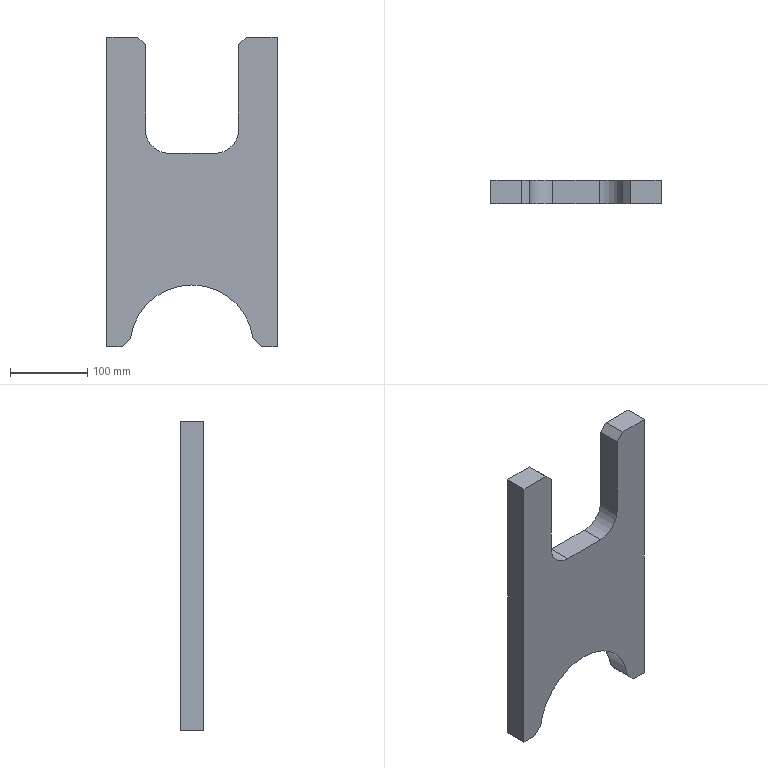Part | SolidWorks | features Chamfer 1, Extrusion 1, Fillet 1 | 1 solid | 18 faces | box 220 x 30 x 400 mm | volume 1803857 mm3 | plane 15 | cylinder 3 | commonest cylinder face diameters 60 x2 160 x1
STEP:
#1=CARTESIAN_POINT('',(110.,0.,200.));
#2=VERTEX_POINT('',#1);
#3=CARTESIAN_POINT('',(110.,0.,-200.));
#4=VERTEX_POINT('',#3);
#5=CARTESIAN_POINT('',(110.,0.,200.));
#6=DIRECTION('',(0.,0.,-1.));
#7=VECTOR('',#6,1000.);
#8=LINE('',#5,#7);
#9=EDGE_CURVE('',#2,#4,#8,.T.);
#10=ORIENTED_EDGE('',*,*,#9,.T.);
#11=CARTESIAN_POINT('',(110.,30.,-200.));
#12=VERTEX_POINT('',#11);
#13=CARTESIAN_POINT('',(110.,30.,-200.));
#14=DIRECTION('',(0.,-1.,0.));
#15=VECTOR('',#14,1000.);
#16=LINE('',#13,#15);
#17=EDGE_CURVE('',#12,#4,#16,.T.);
#18=ORIENTED_EDGE('',*,*,#17,.F.);
#19=CARTESIAN_POINT('',(110.,30.,200.));
#20=VERTEX_POINT('',#19);
#21=CARTESIAN_POINT('',(110.,30.,200.));
#22=DIRECTION('',(0.,0.,-1.));
#23=VECTOR('',#22,1000.);
#24=LINE('',#21,#23);
#25=EDGE_CURVE('',#20,#12,#24,.T.);
#26=ORIENTED_EDGE('',*,*,#25,.F.);
#27=CARTESIAN_POINT('',(110.,30.,200.));
#28=DIRECTION('',(0.,-1.,0.));
#29=VECTOR('',#28,1000.);
#30=LINE('',#27,#29);
#31=EDGE_CURVE('',#20,#2,#30,.T.);
#32=ORIENTED_EDGE('',*,*,#31,.T.);
#33=EDGE_LOOP('',(#10,#18,#26,#32));
#34=FACE_OUTER_BOUND('',#33,.T.);
#35=CARTESIAN_POINT('',(110.,30.,200.));
#36=DIRECTION('',(-1.,0.,0.));
#37=DIRECTION('',(0.,0.,1.));
#38=AXIS2_PLACEMENT_3D('',#35,#36,#37);
#39=PLANE('',#38);
#40=ADVANCED_FACE('',(#34),#39,.F.);
#41=CARTESIAN_POINT('',(89.703,0.,-200.));
#42=VERTEX_POINT('',#41);
#43=CARTESIAN_POINT('',(79.703,0.,-200.));
#44=DIRECTION('',(-1.,0.,0.));
#45=VECTOR('',#44,1000.);
#46=LINE('',#43,#45);
#47=EDGE_CURVE('',#4,#42,#46,.T.);
#48=ORIENTED_EDGE('',*,*,#47,.T.);
#49=CARTESIAN_POINT('',(89.703,30.,-200.));
#50=VERTEX_POINT('',#49);
#51=CARTESIAN_POINT('',(89.703,30.,-200.));
#52=DIRECTION('',(0.,1.,0.));
#53=VECTOR('',#52,1000.);
#54=LINE('',#51,#53);
#55=EDGE_CURVE('',#42,#50,#54,.T.);
#56=ORIENTED_EDGE('',*,*,#55,.T.);
#57=CARTESIAN_POINT('',(79.703,30.,-200.));
#58=DIRECTION('',(-1.,0.,0.));
#59=VECTOR('',#58,1000.);
#60=LINE('',#57,#59);
#61=EDGE_CURVE('',#12,#50,#60,.T.);
#62=ORIENTED_EDGE('',*,*,#61,.F.);
#63=ORIENTED_EDGE('',*,*,#17,.T.);
#64=EDGE_LOOP('',(#48,#56,#62,#63));
#65=FACE_OUTER_BOUND('',#64,.T.);
#66=CARTESIAN_POINT('',(79.703,30.,-200.));
#67=DIRECTION('',(0.,0.,1.));
#68=DIRECTION('',(1.,0.,0.));
#69=AXIS2_PLACEMENT_3D('',#66,#67,#68);
#70=PLANE('',#69);
#71=ADVANCED_FACE('',(#65),#70,.F.);
#72=CARTESIAN_POINT('',(78.981,30.,-189.278));
#73=VERTEX_POINT('',#72);
#74=CARTESIAN_POINT('',(-79.575,30.,-189.278));
#75=VERTEX_POINT('',#74);
#76=CARTESIAN_POINT('',(-0.2969,30.,-200.));
#77=DIRECTION('',(0.,-1.,0.));
#78=DIRECTION('',(0.,0.,1.));
#79=AXIS2_PLACEMENT_3D('',#76,#77,#78);
#80=CIRCLE('',#79,80.);
#81=EDGE_CURVE('',#73,#75,#80,.T.);
#82=ORIENTED_EDGE('',*,*,#81,.F.);
#83=CARTESIAN_POINT('',(78.981,0.,-189.278));
#84=VERTEX_POINT('',#83);
#85=CARTESIAN_POINT('',(78.981,30.,-189.278));
#86=DIRECTION('',(0.,-1.,0.));
#87=VECTOR('',#86,1000.);
#88=LINE('',#85,#87);
#89=EDGE_CURVE('',#73,#84,#88,.T.);
#90=ORIENTED_EDGE('',*,*,#89,.T.);
#91=CARTESIAN_POINT('',(-79.575,0.,-189.278));
#92=VERTEX_POINT('',#91);
#93=CARTESIAN_POINT('',(-0.2969,0.,-200.));
#94=DIRECTION('',(0.,-1.,0.));
#95=DIRECTION('',(0.,0.,1.));
#96=AXIS2_PLACEMENT_3D('',#93,#94,#95);
#97=CIRCLE('',#96,80.);
#98=EDGE_CURVE('',#84,#92,#97,.T.);
#99=ORIENTED_EDGE('',*,*,#98,.T.);
#100=CARTESIAN_POINT('',(-79.575,30.,-189.278));
#101=DIRECTION('',(0.,1.,0.));
#102=VECTOR('',#101,1000.);
#103=LINE('',#100,#102);
#104=EDGE_CURVE('',#92,#75,#103,.T.);
#105=ORIENTED_EDGE('',*,*,#104,.T.);
#106=EDGE_LOOP('',(#82,#90,#99,#105));
#107=FACE_OUTER_BOUND('',#106,.T.);
#108=CARTESIAN_POINT('',(-0.2969,30.,-200.));
#109=DIRECTION('',(0.,-1.,0.));
#110=DIRECTION('',(0.,0.,-1.));
#111=AXIS2_PLACEMENT_3D('',#108,#109,#110);
#112=CYLINDRICAL_SURFACE('',#111,80.);
#113=ADVANCED_FACE('',(#107),#112,.F.);
#114=CARTESIAN_POINT('',(-90.297,30.,-200.));
#115=VERTEX_POINT('',#114);
#116=CARTESIAN_POINT('',(-110.,30.,-200.));
#117=VERTEX_POINT('',#116);
#118=CARTESIAN_POINT('',(-110.,30.,-200.));
#119=DIRECTION('',(-1.,0.,0.));
#120=VECTOR('',#119,1000.);
#121=LINE('',#118,#120);
#122=EDGE_CURVE('',#115,#117,#121,.T.);
#123=ORIENTED_EDGE('',*,*,#122,.F.);
#124=CARTESIAN_POINT('',(-90.297,0.,-200.));
#125=VERTEX_POINT('',#124);
#126=CARTESIAN_POINT('',(-90.297,30.,-200.));
#127=DIRECTION('',(0.,-1.,0.));
#128=VECTOR('',#127,1000.);
#129=LINE('',#126,#128);
#130=EDGE_CURVE('',#115,#125,#129,.T.);
#131=ORIENTED_EDGE('',*,*,#130,.T.);
#132=CARTESIAN_POINT('',(-110.,0.,-200.));
#133=VERTEX_POINT('',#132);
#134=CARTESIAN_POINT('',(-110.,0.,-200.));
#135=DIRECTION('',(-1.,0.,0.));
#136=VECTOR('',#135,1000.);
#137=LINE('',#134,#136);
#138=EDGE_CURVE('',#125,#133,#137,.T.);
#139=ORIENTED_EDGE('',*,*,#138,.T.);
#140=CARTESIAN_POINT('',(-110.,30.,-200.));
#141=DIRECTION('',(0.,-1.,0.));
#142=VECTOR('',#141,1000.);
#143=LINE('',#140,#142);
#144=EDGE_CURVE('',#117,#133,#143,.T.);
#145=ORIENTED_EDGE('',*,*,#144,.F.);
#146=EDGE_LOOP('',(#123,#131,#139,#145));
#147=FACE_OUTER_BOUND('',#146,.T.);
#148=CARTESIAN_POINT('',(-110.,30.,-200.));
#149=DIRECTION('',(0.,0.,1.));
#150=DIRECTION('',(1.,0.,0.));
#151=AXIS2_PLACEMENT_3D('',#148,#149,#150);
#152=PLANE('',#151);
#153=ADVANCED_FACE('',(#147),#152,.F.);
#154=CARTESIAN_POINT('',(-110.,0.,200.));
#155=VERTEX_POINT('',#154);
#156=CARTESIAN_POINT('',(-110.,0.,200.));
#157=DIRECTION('',(0.,0.,1.));
#158=VECTOR('',#157,1000.);
#159=LINE('',#156,#158);
#160=EDGE_CURVE('',#133,#155,#159,.T.);
#161=ORIENTED_EDGE('',*,*,#160,.T.);
#162=CARTESIAN_POINT('',(-110.,30.,200.));
#163=VERTEX_POINT('',#162);
#164=CARTESIAN_POINT('',(-110.,30.,200.));
#165=DIRECTION('',(0.,-1.,0.));
#166=VECTOR('',#165,1000.);
#167=LINE('',#164,#166);
#168=EDGE_CURVE('',#163,#155,#167,.T.);
#169=ORIENTED_EDGE('',*,*,#168,.F.);
#170=CARTESIAN_POINT('',(-110.,30.,200.));
#171=DIRECTION('',(0.,0.,1.));
#172=VECTOR('',#171,1000.);
#173=LINE('',#170,#172);
#174=EDGE_CURVE('',#117,#163,#173,.T.);
#175=ORIENTED_EDGE('',*,*,#174,.F.);
#176=ORIENTED_EDGE('',*,*,#144,.T.);
#177=EDGE_LOOP('',(#161,#169,#175,#176));
#178=FACE_OUTER_BOUND('',#177,.T.);
#179=CARTESIAN_POINT('',(-110.,30.,200.));
#180=DIRECTION('',(1.,0.,0.));
#181=DIRECTION('',(0.,0.,-1.));
#182=AXIS2_PLACEMENT_3D('',#179,#180,#181);
#183=PLANE('',#182);
#184=ADVANCED_FACE('',(#178),#183,.F.);
#185=CARTESIAN_POINT('',(-70.,0.,200.));
#186=VERTEX_POINT('',#185);
#187=CARTESIAN_POINT('',(-110.,0.,200.));
#188=DIRECTION('',(1.,0.,0.));
#189=VECTOR('',#188,1000.);
#190=LINE('',#187,#189);
#191=EDGE_CURVE('',#155,#186,#190,.T.);
#192=ORIENTED_EDGE('',*,*,#191,.T.);
#193=CARTESIAN_POINT('',(-70.,30.,200.));
#194=VERTEX_POINT('',#193);
#195=CARTESIAN_POINT('',(-70.,30.,200.));
#196=DIRECTION('',(0.,1.,0.));
#197=VECTOR('',#196,1000.);
#198=LINE('',#195,#197);
#199=EDGE_CURVE('',#186,#194,#198,.T.);
#200=ORIENTED_EDGE('',*,*,#199,.T.);
#201=CARTESIAN_POINT('',(-110.,30.,200.));
#202=DIRECTION('',(1.,0.,0.));
#203=VECTOR('',#202,1000.);
#204=LINE('',#201,#203);
#205=EDGE_CURVE('',#163,#194,#204,.T.);
#206=ORIENTED_EDGE('',*,*,#205,.F.);
#207=ORIENTED_EDGE('',*,*,#168,.T.);
#208=EDGE_LOOP('',(#192,#200,#206,#207));
#209=FACE_OUTER_BOUND('',#208,.T.);
#210=CARTESIAN_POINT('',(-110.,30.,200.));
#211=DIRECTION('',(0.,0.,-1.));
#212=DIRECTION('',(-1.,0.,0.));
#213=AXIS2_PLACEMENT_3D('',#210,#211,#212);
#214=PLANE('',#213);
#215=ADVANCED_FACE('',(#209),#214,.F.);
#216=CARTESIAN_POINT('',(-60.,30.,190.));
#217=VERTEX_POINT('',#216);
#218=CARTESIAN_POINT('',(-60.,30.,80.));
#219=VERTEX_POINT('',#218);
#220=CARTESIAN_POINT('',(-60.,30.,200.));
#221=DIRECTION('',(0.,0.,-1.));
#222=VECTOR('',#221,1000.);
#223=LINE('',#220,#222);
#224=EDGE_CURVE('',#217,#219,#223,.T.);
#225=ORIENTED_EDGE('',*,*,#224,.F.);
#226=CARTESIAN_POINT('',(-60.,0.,190.));
#227=VERTEX_POINT('',#226);
#228=CARTESIAN_POINT('',(-60.,30.,190.));
#229=DIRECTION('',(0.,-1.,0.));
#230=VECTOR('',#229,1000.);
#231=LINE('',#228,#230);
#232=EDGE_CURVE('',#217,#227,#231,.T.);
#233=ORIENTED_EDGE('',*,*,#232,.T.);
#234=CARTESIAN_POINT('',(-60.,0.,80.));
#235=VERTEX_POINT('',#234);
#236=CARTESIAN_POINT('',(-60.,0.,200.));
#237=DIRECTION('',(0.,0.,-1.));
#238=VECTOR('',#237,1000.);
#239=LINE('',#236,#238);
#240=EDGE_CURVE('',#227,#235,#239,.T.);
#241=ORIENTED_EDGE('',*,*,#240,.T.);
#242=CARTESIAN_POINT('',(-60.,30.,80.));
#243=DIRECTION('',(0.,1.,0.));
#244=VECTOR('',#243,1000.);
#245=LINE('',#242,#244);
#246=EDGE_CURVE('',#235,#219,#245,.T.);
#247=ORIENTED_EDGE('',*,*,#246,.T.);
#248=EDGE_LOOP('',(#225,#233,#241,#247));
#249=FACE_OUTER_BOUND('',#248,.T.);
#250=CARTESIAN_POINT('',(-60.,30.,200.));
#251=DIRECTION('',(-1.,0.,0.));
#252=DIRECTION('',(0.,0.,1.));
#253=AXIS2_PLACEMENT_3D('',#250,#251,#252);
#254=PLANE('',#253);
#255=ADVANCED_FACE('',(#249),#254,.F.);
#256=CARTESIAN_POINT('',(-30.,0.,50.));
#257=VERTEX_POINT('',#256);
#258=CARTESIAN_POINT('',(30.,0.,50.));
#259=VERTEX_POINT('',#258);
#260=CARTESIAN_POINT('',(-60.,0.,50.));
#261=DIRECTION('',(1.,0.,0.));
#262=VECTOR('',#261,1000.);
#263=LINE('',#260,#262);
#264=EDGE_CURVE('',#257,#259,#263,.T.);
#265=ORIENTED_EDGE('',*,*,#264,.T.);
#266=CARTESIAN_POINT('',(30.,30.,50.));
#267=VERTEX_POINT('',#266);
#268=CARTESIAN_POINT('',(30.,30.,50.));
#269=DIRECTION('',(0.,1.,0.));
#270=VECTOR('',#269,1000.);
#271=LINE('',#268,#270);
#272=EDGE_CURVE('',#259,#267,#271,.T.);
#273=ORIENTED_EDGE('',*,*,#272,.T.);
#274=CARTESIAN_POINT('',(-30.,30.,50.));
#275=VERTEX_POINT('',#274);
#276=CARTESIAN_POINT('',(-60.,30.,50.));
#277=DIRECTION('',(1.,0.,0.));
#278=VECTOR('',#277,1000.);
#279=LINE('',#276,#278);
#280=EDGE_CURVE('',#275,#267,#279,.T.);
#281=ORIENTED_EDGE('',*,*,#280,.F.);
#282=CARTESIAN_POINT('',(-30.,0.,50.));
#283=DIRECTION('',(0.,-1.,0.));
#284=VECTOR('',#283,1000.);
#285=LINE('',#282,#284);
#286=EDGE_CURVE('',#275,#257,#285,.T.);
#287=ORIENTED_EDGE('',*,*,#286,.T.);
#288=EDGE_LOOP('',(#265,#273,#281,#287));
#289=FACE_OUTER_BOUND('',#288,.T.);
#290=CARTESIAN_POINT('',(-60.,30.,50.));
#291=DIRECTION('',(0.,0.,-1.));
#292=DIRECTION('',(-1.,0.,0.));
#293=AXIS2_PLACEMENT_3D('',#290,#291,#292);
#294=PLANE('',#293);
#295=ADVANCED_FACE('',(#289),#294,.F.);
#296=CARTESIAN_POINT('',(60.,0.,80.));
#297=VERTEX_POINT('',#296);
#298=CARTESIAN_POINT('',(60.,0.,190.));
#299=VERTEX_POINT('',#298);
#300=CARTESIAN_POINT('',(60.,0.,200.));
#301=DIRECTION('',(0.,0.,1.));
#302=VECTOR('',#301,1000.);
#303=LINE('',#300,#302);
#304=EDGE_CURVE('',#297,#299,#303,.T.);
#305=ORIENTED_EDGE('',*,*,#304,.T.);
#306=CARTESIAN_POINT('',(60.,30.,190.));
#307=VERTEX_POINT('',#306);
#308=CARTESIAN_POINT('',(60.,30.,190.));
#309=DIRECTION('',(0.,1.,0.));
#310=VECTOR('',#309,1000.);
#311=LINE('',#308,#310);
#312=EDGE_CURVE('',#299,#307,#311,.T.);
#313=ORIENTED_EDGE('',*,*,#312,.T.);
#314=CARTESIAN_POINT('',(60.,30.,80.));
#315=VERTEX_POINT('',#314);
#316=CARTESIAN_POINT('',(60.,30.,200.));
#317=DIRECTION('',(0.,0.,1.));
#318=VECTOR('',#317,1000.);
#319=LINE('',#316,#318);
#320=EDGE_CURVE('',#315,#307,#319,.T.);
#321=ORIENTED_EDGE('',*,*,#320,.F.);
#322=CARTESIAN_POINT('',(60.,0.,80.));
#323=DIRECTION('',(0.,-1.,0.));
#324=VECTOR('',#323,1000.);
#325=LINE('',#322,#324);
#326=EDGE_CURVE('',#315,#297,#325,.T.);
#327=ORIENTED_EDGE('',*,*,#326,.T.);
#328=EDGE_LOOP('',(#305,#313,#321,#327));
#329=FACE_OUTER_BOUND('',#328,.T.);
#330=CARTESIAN_POINT('',(60.,30.,200.));
#331=DIRECTION('',(1.,0.,0.));
#332=DIRECTION('',(0.,0.,-1.));
#333=AXIS2_PLACEMENT_3D('',#330,#331,#332);
#334=PLANE('',#333);
#335=ADVANCED_FACE('',(#329),#334,.F.);
#336=CARTESIAN_POINT('',(70.,30.,200.));
#337=VERTEX_POINT('',#336);
#338=CARTESIAN_POINT('',(60.,30.,200.));
#339=DIRECTION('',(1.,0.,0.));
#340=VECTOR('',#339,1000.);
#341=LINE('',#338,#340);
#342=EDGE_CURVE('',#337,#20,#341,.T.);
#343=ORIENTED_EDGE('',*,*,#342,.F.);
#344=CARTESIAN_POINT('',(70.,0.,200.));
#345=VERTEX_POINT('',#344);
#346=CARTESIAN_POINT('',(70.,30.,200.));
#347=DIRECTION('',(0.,-1.,0.));
#348=VECTOR('',#347,1000.);
#349=LINE('',#346,#348);
#350=EDGE_CURVE('',#337,#345,#349,.T.);
#351=ORIENTED_EDGE('',*,*,#350,.T.);
#352=CARTESIAN_POINT('',(60.,0.,200.));
#353=DIRECTION('',(1.,0.,0.));
#354=VECTOR('',#353,1000.);
#355=LINE('',#352,#354);
#356=EDGE_CURVE('',#345,#2,#355,.T.);
#357=ORIENTED_EDGE('',*,*,#356,.T.);
#358=ORIENTED_EDGE('',*,*,#31,.F.);
#359=EDGE_LOOP('',(#343,#351,#357,#358));
#360=FACE_OUTER_BOUND('',#359,.T.);
#361=CARTESIAN_POINT('',(60.,30.,200.));
#362=DIRECTION('',(0.,0.,-1.));
#363=DIRECTION('',(-1.,0.,0.));
#364=AXIS2_PLACEMENT_3D('',#361,#362,#363);
#365=PLANE('',#364);
#366=ADVANCED_FACE('',(#360),#365,.F.);
#367=ORIENTED_EDGE('',*,*,#320,.T.);
#368=CARTESIAN_POINT('',(-165.148,30.,-35.148));
#369=DIRECTION('',(0.7071,0.,0.7071));
#370=VECTOR('',#369,1000.);
#371=LINE('',#368,#370);
#372=EDGE_CURVE('',#307,#337,#371,.T.);
#373=ORIENTED_EDGE('',*,*,#372,.T.);
#374=ORIENTED_EDGE('',*,*,#342,.T.);
#375=ORIENTED_EDGE('',*,*,#25,.T.);
#376=ORIENTED_EDGE('',*,*,#61,.T.);
#377=CARTESIAN_POINT('',(44.703,30.,-155.));
#378=DIRECTION('',(-0.7071,0.,0.7071));
#379=VECTOR('',#378,1000.);
#380=LINE('',#377,#379);
#381=EDGE_CURVE('',#50,#73,#380,.T.);
#382=ORIENTED_EDGE('',*,*,#381,.T.);
#383=ORIENTED_EDGE('',*,*,#81,.T.);
#384=CARTESIAN_POINT('',(-45.297,30.,-155.));
#385=DIRECTION('',(-0.7071,0.,-0.7071));
#386=VECTOR('',#385,1000.);
#387=LINE('',#384,#386);
#388=EDGE_CURVE('',#75,#115,#387,.T.);
#389=ORIENTED_EDGE('',*,*,#388,.T.);
#390=ORIENTED_EDGE('',*,*,#122,.T.);
#391=ORIENTED_EDGE('',*,*,#174,.T.);
#392=ORIENTED_EDGE('',*,*,#205,.T.);
#393=CARTESIAN_POINT('',(164.852,30.,-34.852));
#394=DIRECTION('',(0.7071,0.,-0.7071));
#395=VECTOR('',#394,1000.);
#396=LINE('',#393,#395);
#397=EDGE_CURVE('',#194,#217,#396,.T.);
#398=ORIENTED_EDGE('',*,*,#397,.T.);
#399=ORIENTED_EDGE('',*,*,#224,.T.);
#400=CARTESIAN_POINT('',(-30.,30.,80.));
#401=DIRECTION('',(0.,-1.,0.));
#402=DIRECTION('',(0.,0.,1.));
#403=AXIS2_PLACEMENT_3D('',#400,#401,#402);
#404=CIRCLE('',#403,30.);
#405=EDGE_CURVE('',#219,#275,#404,.T.);
#406=ORIENTED_EDGE('',*,*,#405,.T.);
#407=ORIENTED_EDGE('',*,*,#280,.T.);
#408=CARTESIAN_POINT('',(30.,30.,80.));
#409=DIRECTION('',(0.,-1.,0.));
#410=DIRECTION('',(0.,0.,1.));
#411=AXIS2_PLACEMENT_3D('',#408,#409,#410);
#412=CIRCLE('',#411,30.);
#413=EDGE_CURVE('',#267,#315,#412,.T.);
#414=ORIENTED_EDGE('',*,*,#413,.T.);
#415=EDGE_LOOP('',(#367,#373,#374,#375,#376,#382,#383,#389,#390,#391,#392,#398,#399,#406,#407,#414));
#416=FACE_OUTER_BOUND('',#415,.T.);
#417=CARTESIAN_POINT('',(-0.2969,30.,-200.));
#418=DIRECTION('',(0.,1.,0.));
#419=DIRECTION('',(0.,0.,1.));
#420=AXIS2_PLACEMENT_3D('',#417,#418,#419);
#421=PLANE('',#420);
#422=ADVANCED_FACE('',(#416),#421,.T.);
#423=ORIENTED_EDGE('',*,*,#356,.F.);
#424=CARTESIAN_POINT('',(70.,0.,200.));
#425=DIRECTION('',(-0.7071,0.,-0.7071));
#426=VECTOR('',#425,1000.);
#427=LINE('',#424,#426);
#428=EDGE_CURVE('',#345,#299,#427,.T.);
#429=ORIENTED_EDGE('',*,*,#428,.T.);
#430=ORIENTED_EDGE('',*,*,#304,.F.);
#431=CARTESIAN_POINT('',(30.,0.,80.));
#432=DIRECTION('',(0.,1.,0.));
#433=DIRECTION('',(0.,0.,1.));
#434=AXIS2_PLACEMENT_3D('',#431,#432,#433);
#435=CIRCLE('',#434,30.);
#436=EDGE_CURVE('',#297,#259,#435,.T.);
#437=ORIENTED_EDGE('',*,*,#436,.T.);
#438=ORIENTED_EDGE('',*,*,#264,.F.);
#439=CARTESIAN_POINT('',(-30.,0.,80.));
#440=DIRECTION('',(0.,1.,0.));
#441=DIRECTION('',(0.,0.,1.));
#442=AXIS2_PLACEMENT_3D('',#439,#440,#441);
#443=CIRCLE('',#442,30.);
#444=EDGE_CURVE('',#257,#235,#443,.T.);
#445=ORIENTED_EDGE('',*,*,#444,.T.);
#446=ORIENTED_EDGE('',*,*,#240,.F.);
#447=CARTESIAN_POINT('',(-60.,0.,190.));
#448=DIRECTION('',(-0.7071,0.,0.7071));
#449=VECTOR('',#448,1000.);
#450=LINE('',#447,#449);
#451=EDGE_CURVE('',#227,#186,#450,.T.);
#452=ORIENTED_EDGE('',*,*,#451,.T.);
#453=ORIENTED_EDGE('',*,*,#191,.F.);
#454=ORIENTED_EDGE('',*,*,#160,.F.);
#455=ORIENTED_EDGE('',*,*,#138,.F.);
#456=CARTESIAN_POINT('',(-90.297,0.,-200.));
#457=DIRECTION('',(0.7071,0.,0.7071));
#458=VECTOR('',#457,1000.);
#459=LINE('',#456,#458);
#460=EDGE_CURVE('',#125,#92,#459,.T.);
#461=ORIENTED_EDGE('',*,*,#460,.T.);
#462=ORIENTED_EDGE('',*,*,#98,.F.);
#463=CARTESIAN_POINT('',(78.981,0.,-189.278));
#464=DIRECTION('',(0.7071,0.,-0.7071));
#465=VECTOR('',#464,1000.);
#466=LINE('',#463,#465);
#467=EDGE_CURVE('',#84,#42,#466,.T.);
#468=ORIENTED_EDGE('',*,*,#467,.T.);
#469=ORIENTED_EDGE('',*,*,#47,.F.);
#470=ORIENTED_EDGE('',*,*,#9,.F.);
#471=EDGE_LOOP('',(#423,#429,#430,#437,#438,#445,#446,#452,#453,#454,#455,#461,#462,#468,#469,#470));
#472=FACE_OUTER_BOUND('',#471,.T.);
#473=CARTESIAN_POINT('',(-0.2969,0.,-200.));
#474=DIRECTION('',(0.,1.,0.));
#475=DIRECTION('',(0.,0.,1.));
#476=AXIS2_PLACEMENT_3D('',#473,#474,#475);
#477=PLANE('',#476);
#478=ADVANCED_FACE('',(#472),#477,.F.);
#479=ORIENTED_EDGE('',*,*,#413,.F.);
#480=ORIENTED_EDGE('',*,*,#272,.F.);
#481=ORIENTED_EDGE('',*,*,#436,.F.);
#482=ORIENTED_EDGE('',*,*,#326,.F.);
#483=EDGE_LOOP('',(#479,#480,#481,#482));
#484=FACE_OUTER_BOUND('',#483,.T.);
#485=CARTESIAN_POINT('',(30.,30.,80.));
#486=DIRECTION('',(0.,1.,0.));
#487=DIRECTION('',(0.,0.,1.));
#488=AXIS2_PLACEMENT_3D('',#485,#486,#487);
#489=CYLINDRICAL_SURFACE('',#488,30.);
#490=ADVANCED_FACE('',(#484),#489,.F.);
#491=ORIENTED_EDGE('',*,*,#405,.F.);
#492=ORIENTED_EDGE('',*,*,#246,.F.);
#493=ORIENTED_EDGE('',*,*,#444,.F.);
#494=ORIENTED_EDGE('',*,*,#286,.F.);
#495=EDGE_LOOP('',(#491,#492,#493,#494));
#496=FACE_OUTER_BOUND('',#495,.T.);
#497=CARTESIAN_POINT('',(-30.,30.,80.));
#498=DIRECTION('',(0.,1.,0.));
#499=DIRECTION('',(0.,0.,1.));
#500=AXIS2_PLACEMENT_3D('',#497,#498,#499);
#501=CYLINDRICAL_SURFACE('',#500,30.);
#502=ADVANCED_FACE('',(#496),#501,.F.);
#503=ORIENTED_EDGE('',*,*,#372,.F.);
#504=ORIENTED_EDGE('',*,*,#312,.F.);
#505=ORIENTED_EDGE('',*,*,#428,.F.);
#506=ORIENTED_EDGE('',*,*,#350,.F.);
#507=EDGE_LOOP('',(#503,#504,#505,#506));
#508=FACE_OUTER_BOUND('',#507,.T.);
#509=CARTESIAN_POINT('',(70.,30.,200.));
#510=DIRECTION('',(0.7071,0.,-0.7071));
#511=DIRECTION('',(0.,-1.,0.));
#512=AXIS2_PLACEMENT_3D('',#509,#510,#511);
#513=PLANE('',#512);
#514=ADVANCED_FACE('',(#508),#513,.F.);
#515=ORIENTED_EDGE('',*,*,#397,.F.);
#516=ORIENTED_EDGE('',*,*,#199,.F.);
#517=ORIENTED_EDGE('',*,*,#451,.F.);
#518=ORIENTED_EDGE('',*,*,#232,.F.);
#519=EDGE_LOOP('',(#515,#516,#517,#518));
#520=FACE_OUTER_BOUND('',#519,.T.);
#521=CARTESIAN_POINT('',(-60.,30.,190.));
#522=DIRECTION('',(-0.7071,0.,-0.7071));
#523=DIRECTION('',(0.,-1.,0.));
#524=AXIS2_PLACEMENT_3D('',#521,#522,#523);
#525=PLANE('',#524);
#526=ADVANCED_FACE('',(#520),#525,.F.);
#527=ORIENTED_EDGE('',*,*,#381,.F.);
#528=ORIENTED_EDGE('',*,*,#55,.F.);
#529=ORIENTED_EDGE('',*,*,#467,.F.);
#530=ORIENTED_EDGE('',*,*,#89,.F.);
#531=EDGE_LOOP('',(#527,#528,#529,#530));
#532=FACE_OUTER_BOUND('',#531,.T.);
#533=CARTESIAN_POINT('',(78.981,30.,-189.278));
#534=DIRECTION('',(0.7071,0.,0.7071));
#535=DIRECTION('',(0.,-1.,0.));
#536=AXIS2_PLACEMENT_3D('',#533,#534,#535);
#537=PLANE('',#536);
#538=ADVANCED_FACE('',(#532),#537,.F.);
#539=ORIENTED_EDGE('',*,*,#388,.F.);
#540=ORIENTED_EDGE('',*,*,#104,.F.);
#541=ORIENTED_EDGE('',*,*,#460,.F.);
#542=ORIENTED_EDGE('',*,*,#130,.F.);
#543=EDGE_LOOP('',(#539,#540,#541,#542));
#544=FACE_OUTER_BOUND('',#543,.T.);
#545=CARTESIAN_POINT('',(-90.297,30.,-200.));
#546=DIRECTION('',(-0.7071,0.,0.7071));
#547=DIRECTION('',(0.,-1.,0.));
#548=AXIS2_PLACEMENT_3D('',#545,#546,#547);
#549=PLANE('',#548);
#550=ADVANCED_FACE('',(#544),#549,.F.);
#551=CLOSED_SHELL('',(#40,#71,#113,#153,#184,#215,#255,#295,#335,#366,#422,#478,#490,#502,#514,#526,#538,#550));
#552=MANIFOLD_SOLID_BREP('',#551);
#553=CARTESIAN_POINT('',(0.,0.,0.));
#554=DIRECTION('',(0.,0.,1.));
#555=DIRECTION('',(1.,0.,0.));
#556=AXIS2_PLACEMENT_3D('',#553,#554,#555);
#557=(LENGTH_UNIT()NAMED_UNIT(*)SI_UNIT(.MILLI.,.METRE.));
#558=UNCERTAINTY_MEASURE_WITH_UNIT(LENGTH_MEASURE(0.00001),#557,'','');
#559=(NAMED_UNIT(*)PLANE_ANGLE_UNIT()SI_UNIT($,.RADIAN.));
#560=(NAMED_UNIT(*)SI_UNIT($,.STERADIAN.)SOLID_ANGLE_UNIT());
#561=(GEOMETRIC_REPRESENTATION_CONTEXT(3)GLOBAL_UNCERTAINTY_ASSIGNED_CONTEXT((#558))GLOBAL_UNIT_ASSIGNED_CONTEXT((#557,#559,#560))REPRESENTATION_CONTEXT('',''));
#562=ADVANCED_BREP_SHAPE_REPRESENTATION('',(#552,#556),#561);